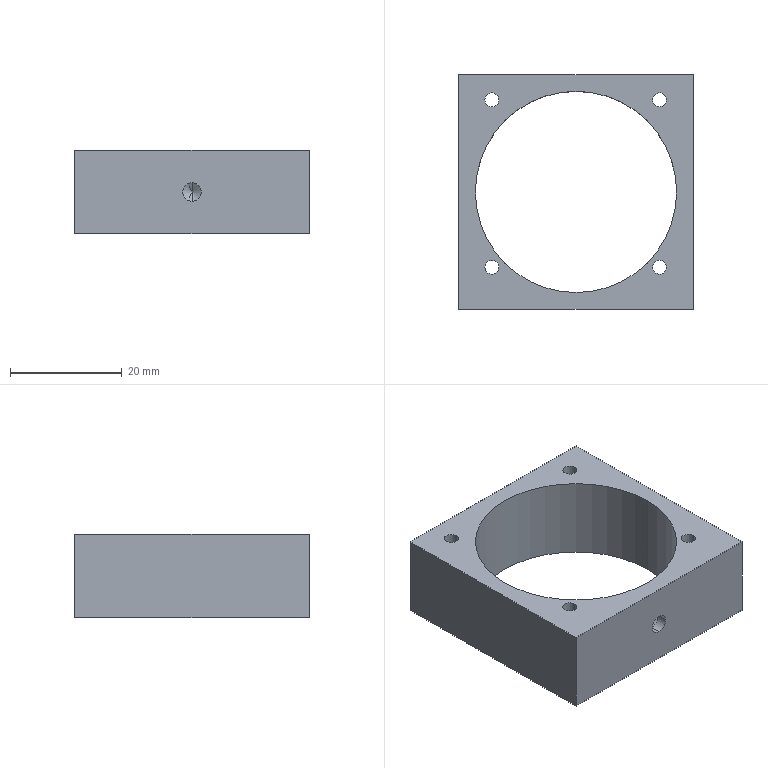Part | STEP file | custom lens barrel.step.STEP.STEP.STEP-260.STEP | 1 solid | 20 faces | box 42 x 42 x 15 mm | volume 10879 mm3 | cylinder 12 | plane 6 | cone 2 | commonest cylinder face diameters 2.5 x8 3.3 x2 36 x2
STEP:
#1=CARTESIAN_POINT('',(0.,-19.2,9.15));
#2=VERTEX_POINT('',#1);
#3=CARTESIAN_POINT('',(0.,-21.,9.15));
#4=VERTEX_POINT('',#3);
#5=CARTESIAN_POINT('',(0.,-21.,9.15));
#6=DIRECTION('',(0.,-1.,0.));
#7=VECTOR('',#6,1000.);
#8=LINE('',#5,#7);
#9=EDGE_CURVE('',#2,#4,#8,.T.);
#10=ORIENTED_EDGE('',*,*,#9,.F.);
#11=CARTESIAN_POINT('',(0.,-19.2,5.85));
#12=VERTEX_POINT('',#11);
#13=CARTESIAN_POINT('',(0.,-19.2,7.5));
#14=DIRECTION('',(0.,-1.,0.));
#15=DIRECTION('',(0.,0.,-1.));
#16=AXIS2_PLACEMENT_3D('',#13,#14,#15);
#17=CIRCLE('',#16,1.65);
#18=EDGE_CURVE('',#12,#2,#17,.T.);
#19=ORIENTED_EDGE('',*,*,#18,.F.);
#20=CARTESIAN_POINT('',(0.,-21.,5.85));
#21=VERTEX_POINT('',#20);
#22=CARTESIAN_POINT('',(0.,-21.,5.85));
#23=DIRECTION('',(0.,-1.,0.));
#24=VECTOR('',#23,1000.);
#25=LINE('',#22,#24);
#26=EDGE_CURVE('',#12,#21,#25,.T.);
#27=ORIENTED_EDGE('',*,*,#26,.T.);
#28=CARTESIAN_POINT('',(0.,-21.,7.5));
#29=DIRECTION('',(0.,-1.,0.));
#30=DIRECTION('',(0.,0.,-1.));
#31=AXIS2_PLACEMENT_3D('',#28,#29,#30);
#32=CIRCLE('',#31,1.65);
#33=EDGE_CURVE('',#21,#4,#32,.T.);
#34=ORIENTED_EDGE('',*,*,#33,.T.);
#35=EDGE_LOOP('',(#10,#19,#27,#34));
#36=FACE_OUTER_BOUND('',#35,.T.);
#37=CARTESIAN_POINT('',(0.,-21.,7.5));
#38=DIRECTION('',(0.,-1.,0.));
#39=DIRECTION('',(0.,0.,-1.));
#40=AXIS2_PLACEMENT_3D('',#37,#38,#39);
#41=CYLINDRICAL_SURFACE('',#40,1.65);
#42=ADVANCED_FACE('',(#36),#41,.F.);
#43=CARTESIAN_POINT('',(0.,-18.209,7.5));
#44=VERTEX_POINT('',#43);
#45=CARTESIAN_POINT('',(0.,-19.2,9.15));
#46=DIRECTION('',(0.,-0.515,0.8572));
#47=VECTOR('',#46,1000.);
#48=LINE('',#45,#47);
#49=EDGE_CURVE('',#44,#2,#48,.T.);
#50=ORIENTED_EDGE('',*,*,#49,.F.);
#51=CARTESIAN_POINT('',(0.,-19.2,5.85));
#52=DIRECTION('',(0.,-0.515,-0.8572));
#53=VECTOR('',#52,1000.);
#54=LINE('',#51,#53);
#55=EDGE_CURVE('',#44,#12,#54,.T.);
#56=ORIENTED_EDGE('',*,*,#55,.T.);
#57=ORIENTED_EDGE('',*,*,#18,.T.);
#58=EDGE_LOOP('',(#50,#56,#57));
#59=FACE_OUTER_BOUND('',#58,.T.);
#60=CARTESIAN_POINT('',(0.,-19.2,7.5));
#61=DIRECTION('',(0.,-1.,0.));
#62=DIRECTION('',(0.,0.,-1.));
#63=AXIS2_PLACEMENT_3D('',#60,#61,#62);
#64=CONICAL_SURFACE('',#63,1.65,1.03);
#65=ADVANCED_FACE('',(#59),#64,.F.);
#66=CARTESIAN_POINT('',(-16.304,16.486,0.));
#67=VERTEX_POINT('',#66);
#68=CARTESIAN_POINT('',(-16.304,16.486,15.));
#69=VERTEX_POINT('',#68);
#70=CARTESIAN_POINT('',(-16.304,16.486,15.));
#71=DIRECTION('',(0.,0.,1.));
#72=VECTOR('',#71,1000.);
#73=LINE('',#70,#72);
#74=EDGE_CURVE('',#67,#69,#73,.T.);
#75=ORIENTED_EDGE('',*,*,#74,.F.);
#76=CARTESIAN_POINT('',(-13.804,16.486,0.));
#77=VERTEX_POINT('',#76);
#78=CARTESIAN_POINT('',(-15.054,16.486,0.));
#79=DIRECTION('',(0.,0.,1.));
#80=DIRECTION('',(1.,0.,0.));
#81=AXIS2_PLACEMENT_3D('',#78,#79,#80);
#82=CIRCLE('',#81,1.25);
#83=EDGE_CURVE('',#77,#67,#82,.T.);
#84=ORIENTED_EDGE('',*,*,#83,.F.);
#85=CARTESIAN_POINT('',(-13.804,16.486,15.));
#86=VERTEX_POINT('',#85);
#87=CARTESIAN_POINT('',(-13.804,16.486,15.));
#88=DIRECTION('',(0.,0.,1.));
#89=VECTOR('',#88,1000.);
#90=LINE('',#87,#89);
#91=EDGE_CURVE('',#77,#86,#90,.T.);
#92=ORIENTED_EDGE('',*,*,#91,.T.);
#93=CARTESIAN_POINT('',(-15.054,16.486,15.));
#94=DIRECTION('',(0.,0.,1.));
#95=DIRECTION('',(1.,0.,0.));
#96=AXIS2_PLACEMENT_3D('',#93,#94,#95);
#97=CIRCLE('',#96,1.25);
#98=EDGE_CURVE('',#86,#69,#97,.T.);
#99=ORIENTED_EDGE('',*,*,#98,.T.);
#100=EDGE_LOOP('',(#75,#84,#92,#99));
#101=FACE_OUTER_BOUND('',#100,.T.);
#102=CARTESIAN_POINT('',(-15.054,16.486,15.));
#103=DIRECTION('',(0.,0.,1.));
#104=DIRECTION('',(1.,0.,0.));
#105=AXIS2_PLACEMENT_3D('',#102,#103,#104);
#106=CYLINDRICAL_SURFACE('',#105,1.25);
#107=ADVANCED_FACE('',(#101),#106,.F.);
#108=CARTESIAN_POINT('',(13.7,16.486,0.));
#109=VERTEX_POINT('',#108);
#110=CARTESIAN_POINT('',(13.7,16.486,15.));
#111=VERTEX_POINT('',#110);
#112=CARTESIAN_POINT('',(13.7,16.486,15.));
#113=DIRECTION('',(0.,0.,1.));
#114=VECTOR('',#113,1000.);
#115=LINE('',#112,#114);
#116=EDGE_CURVE('',#109,#111,#115,.T.);
#117=ORIENTED_EDGE('',*,*,#116,.F.);
#118=CARTESIAN_POINT('',(16.2,16.486,0.));
#119=VERTEX_POINT('',#118);
#120=CARTESIAN_POINT('',(14.95,16.486,0.));
#121=DIRECTION('',(0.,0.,1.));
#122=DIRECTION('',(1.,0.,0.));
#123=AXIS2_PLACEMENT_3D('',#120,#121,#122);
#124=CIRCLE('',#123,1.25);
#125=EDGE_CURVE('',#119,#109,#124,.T.);
#126=ORIENTED_EDGE('',*,*,#125,.F.);
#127=CARTESIAN_POINT('',(16.2,16.486,15.));
#128=VERTEX_POINT('',#127);
#129=CARTESIAN_POINT('',(16.2,16.486,15.));
#130=DIRECTION('',(0.,0.,1.));
#131=VECTOR('',#130,1000.);
#132=LINE('',#129,#131);
#133=EDGE_CURVE('',#119,#128,#132,.T.);
#134=ORIENTED_EDGE('',*,*,#133,.T.);
#135=CARTESIAN_POINT('',(14.95,16.486,15.));
#136=DIRECTION('',(0.,0.,1.));
#137=DIRECTION('',(1.,0.,0.));
#138=AXIS2_PLACEMENT_3D('',#135,#136,#137);
#139=CIRCLE('',#138,1.25);
#140=EDGE_CURVE('',#128,#111,#139,.T.);
#141=ORIENTED_EDGE('',*,*,#140,.T.);
#142=EDGE_LOOP('',(#117,#126,#134,#141));
#143=FACE_OUTER_BOUND('',#142,.T.);
#144=CARTESIAN_POINT('',(14.95,16.486,15.));
#145=DIRECTION('',(0.,0.,1.));
#146=DIRECTION('',(1.,0.,0.));
#147=AXIS2_PLACEMENT_3D('',#144,#145,#146);
#148=CYLINDRICAL_SURFACE('',#147,1.25);
#149=ADVANCED_FACE('',(#143),#148,.F.);
#150=CARTESIAN_POINT('',(13.7,-13.48,0.));
#151=VERTEX_POINT('',#150);
#152=CARTESIAN_POINT('',(13.7,-13.48,15.));
#153=VERTEX_POINT('',#152);
#154=CARTESIAN_POINT('',(13.7,-13.48,15.));
#155=DIRECTION('',(0.,0.,1.));
#156=VECTOR('',#155,1000.);
#157=LINE('',#154,#156);
#158=EDGE_CURVE('',#151,#153,#157,.T.);
#159=ORIENTED_EDGE('',*,*,#158,.F.);
#160=CARTESIAN_POINT('',(16.2,-13.48,0.));
#161=VERTEX_POINT('',#160);
#162=CARTESIAN_POINT('',(14.95,-13.48,0.));
#163=DIRECTION('',(0.,0.,1.));
#164=DIRECTION('',(1.,0.,0.));
#165=AXIS2_PLACEMENT_3D('',#162,#163,#164);
#166=CIRCLE('',#165,1.25);
#167=EDGE_CURVE('',#161,#151,#166,.T.);
#168=ORIENTED_EDGE('',*,*,#167,.F.);
#169=CARTESIAN_POINT('',(16.2,-13.48,15.));
#170=VERTEX_POINT('',#169);
#171=CARTESIAN_POINT('',(16.2,-13.48,15.));
#172=DIRECTION('',(0.,0.,1.));
#173=VECTOR('',#172,1000.);
#174=LINE('',#171,#173);
#175=EDGE_CURVE('',#161,#170,#174,.T.);
#176=ORIENTED_EDGE('',*,*,#175,.T.);
#177=CARTESIAN_POINT('',(14.95,-13.48,15.));
#178=DIRECTION('',(0.,0.,1.));
#179=DIRECTION('',(1.,0.,0.));
#180=AXIS2_PLACEMENT_3D('',#177,#178,#179);
#181=CIRCLE('',#180,1.25);
#182=EDGE_CURVE('',#170,#153,#181,.T.);
#183=ORIENTED_EDGE('',*,*,#182,.T.);
#184=EDGE_LOOP('',(#159,#168,#176,#183));
#185=FACE_OUTER_BOUND('',#184,.T.);
#186=CARTESIAN_POINT('',(14.95,-13.48,15.));
#187=DIRECTION('',(0.,0.,1.));
#188=DIRECTION('',(1.,0.,0.));
#189=AXIS2_PLACEMENT_3D('',#186,#187,#188);
#190=CYLINDRICAL_SURFACE('',#189,1.25);
#191=ADVANCED_FACE('',(#185),#190,.F.);
#192=CARTESIAN_POINT('',(-16.304,-13.48,0.));
#193=VERTEX_POINT('',#192);
#194=CARTESIAN_POINT('',(-16.304,-13.48,15.));
#195=VERTEX_POINT('',#194);
#196=CARTESIAN_POINT('',(-16.304,-13.48,15.));
#197=DIRECTION('',(0.,0.,1.));
#198=VECTOR('',#197,1000.);
#199=LINE('',#196,#198);
#200=EDGE_CURVE('',#193,#195,#199,.T.);
#201=ORIENTED_EDGE('',*,*,#200,.F.);
#202=CARTESIAN_POINT('',(-13.804,-13.48,0.));
#203=VERTEX_POINT('',#202);
#204=CARTESIAN_POINT('',(-15.054,-13.48,0.));
#205=DIRECTION('',(0.,0.,1.));
#206=DIRECTION('',(1.,0.,0.));
#207=AXIS2_PLACEMENT_3D('',#204,#205,#206);
#208=CIRCLE('',#207,1.25);
#209=EDGE_CURVE('',#203,#193,#208,.T.);
#210=ORIENTED_EDGE('',*,*,#209,.F.);
#211=CARTESIAN_POINT('',(-13.804,-13.48,15.));
#212=VERTEX_POINT('',#211);
#213=CARTESIAN_POINT('',(-13.804,-13.48,15.));
#214=DIRECTION('',(0.,0.,1.));
#215=VECTOR('',#214,1000.);
#216=LINE('',#213,#215);
#217=EDGE_CURVE('',#203,#212,#216,.T.);
#218=ORIENTED_EDGE('',*,*,#217,.T.);
#219=CARTESIAN_POINT('',(-15.054,-13.48,15.));
#220=DIRECTION('',(0.,0.,1.));
#221=DIRECTION('',(1.,0.,0.));
#222=AXIS2_PLACEMENT_3D('',#219,#220,#221);
#223=CIRCLE('',#222,1.25);
#224=EDGE_CURVE('',#212,#195,#223,.T.);
#225=ORIENTED_EDGE('',*,*,#224,.T.);
#226=EDGE_LOOP('',(#201,#210,#218,#225));
#227=FACE_OUTER_BOUND('',#226,.T.);
#228=CARTESIAN_POINT('',(-15.054,-13.48,15.));
#229=DIRECTION('',(0.,0.,1.));
#230=DIRECTION('',(1.,0.,0.));
#231=AXIS2_PLACEMENT_3D('',#228,#229,#230);
#232=CYLINDRICAL_SURFACE('',#231,1.25);
#233=ADVANCED_FACE('',(#227),#232,.F.);
#234=CARTESIAN_POINT('',(-18.,0.,0.));
#235=VERTEX_POINT('',#234);
#236=CARTESIAN_POINT('',(18.,0.,0.));
#237=VERTEX_POINT('',#236);
#238=CARTESIAN_POINT('',(0.,0.,0.));
#239=DIRECTION('',(0.,0.,1.));
#240=DIRECTION('',(1.,0.,0.));
#241=AXIS2_PLACEMENT_3D('',#238,#239,#240);
#242=CIRCLE('',#241,18.);
#243=EDGE_CURVE('',#235,#237,#242,.T.);
#244=ORIENTED_EDGE('',*,*,#243,.T.);
#245=CARTESIAN_POINT('',(0.,0.,0.));
#246=DIRECTION('',(0.,0.,1.));
#247=DIRECTION('',(1.,0.,0.));
#248=AXIS2_PLACEMENT_3D('',#245,#246,#247);
#249=CIRCLE('',#248,18.);
#250=EDGE_CURVE('',#237,#235,#249,.T.);
#251=ORIENTED_EDGE('',*,*,#250,.T.);
#252=EDGE_LOOP('',(#244,#251));
#253=FACE_BOUND('',#252,.T.);
#254=ORIENTED_EDGE('',*,*,#209,.T.);
#255=CARTESIAN_POINT('',(-15.054,-13.48,0.));
#256=DIRECTION('',(0.,0.,1.));
#257=DIRECTION('',(1.,0.,0.));
#258=AXIS2_PLACEMENT_3D('',#255,#256,#257);
#259=CIRCLE('',#258,1.25);
#260=EDGE_CURVE('',#193,#203,#259,.T.);
#261=ORIENTED_EDGE('',*,*,#260,.T.);
#262=EDGE_LOOP('',(#254,#261));
#263=FACE_BOUND('',#262,.T.);
#264=ORIENTED_EDGE('',*,*,#167,.T.);
#265=CARTESIAN_POINT('',(14.95,-13.48,0.));
#266=DIRECTION('',(0.,0.,1.));
#267=DIRECTION('',(1.,0.,0.));
#268=AXIS2_PLACEMENT_3D('',#265,#266,#267);
#269=CIRCLE('',#268,1.25);
#270=EDGE_CURVE('',#151,#161,#269,.T.);
#271=ORIENTED_EDGE('',*,*,#270,.T.);
#272=EDGE_LOOP('',(#264,#271));
#273=FACE_BOUND('',#272,.T.);
#274=ORIENTED_EDGE('',*,*,#125,.T.);
#275=CARTESIAN_POINT('',(14.95,16.486,0.));
#276=DIRECTION('',(0.,0.,1.));
#277=DIRECTION('',(1.,0.,0.));
#278=AXIS2_PLACEMENT_3D('',#275,#276,#277);
#279=CIRCLE('',#278,1.25);
#280=EDGE_CURVE('',#109,#119,#279,.T.);
#281=ORIENTED_EDGE('',*,*,#280,.T.);
#282=EDGE_LOOP('',(#274,#281));
#283=FACE_BOUND('',#282,.T.);
#284=ORIENTED_EDGE('',*,*,#83,.T.);
#285=CARTESIAN_POINT('',(-15.054,16.486,0.));
#286=DIRECTION('',(0.,0.,1.));
#287=DIRECTION('',(1.,0.,0.));
#288=AXIS2_PLACEMENT_3D('',#285,#286,#287);
#289=CIRCLE('',#288,1.25);
#290=EDGE_CURVE('',#67,#77,#289,.T.);
#291=ORIENTED_EDGE('',*,*,#290,.T.);
#292=EDGE_LOOP('',(#284,#291));
#293=FACE_BOUND('',#292,.T.);
#294=CARTESIAN_POINT('',(21.,21.,0.));
#295=VERTEX_POINT('',#294);
#296=CARTESIAN_POINT('',(21.,-21.,0.));
#297=VERTEX_POINT('',#296);
#298=CARTESIAN_POINT('',(21.,0.,0.));
#299=DIRECTION('',(0.,-1.,0.));
#300=VECTOR('',#299,1000.);
#301=LINE('',#298,#300);
#302=EDGE_CURVE('',#295,#297,#301,.T.);
#303=ORIENTED_EDGE('',*,*,#302,.T.);
#304=CARTESIAN_POINT('',(-21.,-21.,0.));
#305=VERTEX_POINT('',#304);
#306=CARTESIAN_POINT('',(0.,-21.,0.));
#307=DIRECTION('',(1.,0.,0.));
#308=VECTOR('',#307,1000.);
#309=LINE('',#306,#308);
#310=EDGE_CURVE('',#305,#297,#309,.T.);
#311=ORIENTED_EDGE('',*,*,#310,.F.);
#312=CARTESIAN_POINT('',(-21.,21.,0.));
#313=VERTEX_POINT('',#312);
#314=CARTESIAN_POINT('',(-21.,0.,0.));
#315=DIRECTION('',(0.,-1.,0.));
#316=VECTOR('',#315,1000.);
#317=LINE('',#314,#316);
#318=EDGE_CURVE('',#313,#305,#317,.T.);
#319=ORIENTED_EDGE('',*,*,#318,.F.);
#320=CARTESIAN_POINT('',(0.,21.,0.));
#321=DIRECTION('',(1.,0.,0.));
#322=VECTOR('',#321,1000.);
#323=LINE('',#320,#322);
#324=EDGE_CURVE('',#313,#295,#323,.T.);
#325=ORIENTED_EDGE('',*,*,#324,.T.);
#326=EDGE_LOOP('',(#303,#311,#319,#325));
#327=FACE_OUTER_BOUND('',#326,.T.);
#328=CARTESIAN_POINT('',(0.,0.,0.));
#329=DIRECTION('',(0.,0.,1.));
#330=DIRECTION('',(1.,0.,0.));
#331=AXIS2_PLACEMENT_3D('',#328,#329,#330);
#332=PLANE('',#331);
#333=ADVANCED_FACE('',(#253,#263,#273,#283,#293,#327),#332,.F.);
#334=CARTESIAN_POINT('',(-18.,0.,15.));
#335=VERTEX_POINT('',#334);
#336=CARTESIAN_POINT('',(18.,0.,15.));
#337=VERTEX_POINT('',#336);
#338=CARTESIAN_POINT('',(0.,0.,15.));
#339=DIRECTION('',(0.,0.,1.));
#340=DIRECTION('',(1.,0.,0.));
#341=AXIS2_PLACEMENT_3D('',#338,#339,#340);
#342=CIRCLE('',#341,18.);
#343=EDGE_CURVE('',#335,#337,#342,.T.);
#344=ORIENTED_EDGE('',*,*,#343,.F.);
#345=CARTESIAN_POINT('',(0.,0.,15.));
#346=DIRECTION('',(0.,0.,1.));
#347=DIRECTION('',(1.,0.,0.));
#348=AXIS2_PLACEMENT_3D('',#345,#346,#347);
#349=CIRCLE('',#348,18.);
#350=EDGE_CURVE('',#337,#335,#349,.T.);
#351=ORIENTED_EDGE('',*,*,#350,.F.);
#352=EDGE_LOOP('',(#344,#351));
#353=FACE_BOUND('',#352,.T.);
#354=ORIENTED_EDGE('',*,*,#224,.F.);
#355=CARTESIAN_POINT('',(-15.054,-13.48,15.));
#356=DIRECTION('',(0.,0.,1.));
#357=DIRECTION('',(1.,0.,0.));
#358=AXIS2_PLACEMENT_3D('',#355,#356,#357);
#359=CIRCLE('',#358,1.25);
#360=EDGE_CURVE('',#195,#212,#359,.T.);
#361=ORIENTED_EDGE('',*,*,#360,.F.);
#362=EDGE_LOOP('',(#354,#361));
#363=FACE_BOUND('',#362,.T.);
#364=ORIENTED_EDGE('',*,*,#182,.F.);
#365=CARTESIAN_POINT('',(14.95,-13.48,15.));
#366=DIRECTION('',(0.,0.,1.));
#367=DIRECTION('',(1.,0.,0.));
#368=AXIS2_PLACEMENT_3D('',#365,#366,#367);
#369=CIRCLE('',#368,1.25);
#370=EDGE_CURVE('',#153,#170,#369,.T.);
#371=ORIENTED_EDGE('',*,*,#370,.F.);
#372=EDGE_LOOP('',(#364,#371));
#373=FACE_BOUND('',#372,.T.);
#374=ORIENTED_EDGE('',*,*,#140,.F.);
#375=CARTESIAN_POINT('',(14.95,16.486,15.));
#376=DIRECTION('',(0.,0.,1.));
#377=DIRECTION('',(1.,0.,0.));
#378=AXIS2_PLACEMENT_3D('',#375,#376,#377);
#379=CIRCLE('',#378,1.25);
#380=EDGE_CURVE('',#111,#128,#379,.T.);
#381=ORIENTED_EDGE('',*,*,#380,.F.);
#382=EDGE_LOOP('',(#374,#381));
#383=FACE_BOUND('',#382,.T.);
#384=ORIENTED_EDGE('',*,*,#98,.F.);
#385=CARTESIAN_POINT('',(-15.054,16.486,15.));
#386=DIRECTION('',(0.,0.,1.));
#387=DIRECTION('',(1.,0.,0.));
#388=AXIS2_PLACEMENT_3D('',#385,#386,#387);
#389=CIRCLE('',#388,1.25);
#390=EDGE_CURVE('',#69,#86,#389,.T.);
#391=ORIENTED_EDGE('',*,*,#390,.F.);
#392=EDGE_LOOP('',(#384,#391));
#393=FACE_BOUND('',#392,.T.);
#394=CARTESIAN_POINT('',(21.,21.,15.));
#395=VERTEX_POINT('',#394);
#396=CARTESIAN_POINT('',(21.,-21.,15.));
#397=VERTEX_POINT('',#396);
#398=CARTESIAN_POINT('',(21.,0.,15.));
#399=DIRECTION('',(0.,-1.,0.));
#400=VECTOR('',#399,1000.);
#401=LINE('',#398,#400);
#402=EDGE_CURVE('',#395,#397,#401,.T.);
#403=ORIENTED_EDGE('',*,*,#402,.F.);
#404=CARTESIAN_POINT('',(-21.,21.,15.));
#405=VERTEX_POINT('',#404);
#406=CARTESIAN_POINT('',(0.,21.,15.));
#407=DIRECTION('',(1.,0.,0.));
#408=VECTOR('',#407,1000.);
#409=LINE('',#406,#408);
#410=EDGE_CURVE('',#405,#395,#409,.T.);
#411=ORIENTED_EDGE('',*,*,#410,.F.);
#412=CARTESIAN_POINT('',(-21.,-21.,15.));
#413=VERTEX_POINT('',#412);
#414=CARTESIAN_POINT('',(-21.,0.,15.));
#415=DIRECTION('',(0.,-1.,0.));
#416=VECTOR('',#415,1000.);
#417=LINE('',#414,#416);
#418=EDGE_CURVE('',#405,#413,#417,.T.);
#419=ORIENTED_EDGE('',*,*,#418,.T.);
#420=CARTESIAN_POINT('',(0.,-21.,15.));
#421=DIRECTION('',(1.,0.,0.));
#422=VECTOR('',#421,1000.);
#423=LINE('',#420,#422);
#424=EDGE_CURVE('',#413,#397,#423,.T.);
#425=ORIENTED_EDGE('',*,*,#424,.T.);
#426=EDGE_LOOP('',(#403,#411,#419,#425));
#427=FACE_OUTER_BOUND('',#426,.T.);
#428=CARTESIAN_POINT('',(0.,0.,15.));
#429=DIRECTION('',(0.,0.,1.));
#430=DIRECTION('',(1.,0.,0.));
#431=AXIS2_PLACEMENT_3D('',#428,#429,#430);
#432=PLANE('',#431);
#433=ADVANCED_FACE('',(#353,#363,#373,#383,#393,#427),#432,.T.);
#434=ORIENTED_EDGE('',*,*,#33,.F.);
#435=CARTESIAN_POINT('',(0.,-21.,7.5));
#436=DIRECTION('',(0.,-1.,0.));
#437=DIRECTION('',(0.,0.,-1.));
#438=AXIS2_PLACEMENT_3D('',#435,#436,#437);
#439=CIRCLE('',#438,1.65);
#440=EDGE_CURVE('',#4,#21,#439,.T.);
#441=ORIENTED_EDGE('',*,*,#440,.F.);
#442=EDGE_LOOP('',(#434,#441));
#443=FACE_BOUND('',#442,.T.);
#444=ORIENTED_EDGE('',*,*,#310,.T.);
#445=CARTESIAN_POINT('',(21.,-21.,15.));
#446=DIRECTION('',(0.,0.,-1.));
#447=VECTOR('',#446,1000.);
#448=LINE('',#445,#447);
#449=EDGE_CURVE('',#397,#297,#448,.T.);
#450=ORIENTED_EDGE('',*,*,#449,.F.);
#451=ORIENTED_EDGE('',*,*,#424,.F.);
#452=CARTESIAN_POINT('',(-21.,-21.,15.));
#453=DIRECTION('',(0.,0.,-1.));
#454=VECTOR('',#453,1000.);
#455=LINE('',#452,#454);
#456=EDGE_CURVE('',#413,#305,#455,.T.);
#457=ORIENTED_EDGE('',*,*,#456,.T.);
#458=EDGE_LOOP('',(#444,#450,#451,#457));
#459=FACE_OUTER_BOUND('',#458,.T.);
#460=CARTESIAN_POINT('',(0.,-21.,15.));
#461=DIRECTION('',(0.,1.,0.));
#462=DIRECTION('',(1.,0.,0.));
#463=AXIS2_PLACEMENT_3D('',#460,#461,#462);
#464=PLANE('',#463);
#465=ADVANCED_FACE('',(#443,#459),#464,.F.);
#466=CARTESIAN_POINT('',(18.,0.,15.));
#467=DIRECTION('',(0.,0.,-1.));
#468=VECTOR('',#467,1000.);
#469=LINE('',#466,#468);
#470=EDGE_CURVE('',#337,#237,#469,.T.);
#471=ORIENTED_EDGE('',*,*,#470,.F.);
#472=ORIENTED_EDGE('',*,*,#350,.T.);
#473=CARTESIAN_POINT('',(-18.,0.,15.));
#474=DIRECTION('',(0.,0.,-1.));
#475=VECTOR('',#474,1000.);
#476=LINE('',#473,#475);
#477=EDGE_CURVE('',#335,#235,#476,.T.);
#478=ORIENTED_EDGE('',*,*,#477,.T.);
#479=ORIENTED_EDGE('',*,*,#250,.F.);
#480=EDGE_LOOP('',(#471,#472,#478,#479));
#481=FACE_OUTER_BOUND('',#480,.T.);
#482=CARTESIAN_POINT('',(0.,0.,15.));
#483=DIRECTION('',(0.,0.,-1.));
#484=DIRECTION('',(-1.,0.,0.));
#485=AXIS2_PLACEMENT_3D('',#482,#483,#484);
#486=CYLINDRICAL_SURFACE('',#485,18.);
#487=ADVANCED_FACE('',(#481),#486,.F.);
#488=ORIENTED_EDGE('',*,*,#318,.T.);
#489=ORIENTED_EDGE('',*,*,#456,.F.);
#490=ORIENTED_EDGE('',*,*,#418,.F.);
#491=CARTESIAN_POINT('',(-21.,21.,15.));
#492=DIRECTION('',(0.,0.,-1.));
#493=VECTOR('',#492,1000.);
#494=LINE('',#491,#493);
#495=EDGE_CURVE('',#405,#313,#494,.T.);
#496=ORIENTED_EDGE('',*,*,#495,.T.);
#497=EDGE_LOOP('',(#488,#489,#490,#496));
#498=FACE_OUTER_BOUND('',#497,.T.);
#499=CARTESIAN_POINT('',(-21.,0.,15.));
#500=DIRECTION('',(1.,0.,0.));
#501=DIRECTION('',(0.,1.,0.));
#502=AXIS2_PLACEMENT_3D('',#499,#500,#501);
#503=PLANE('',#502);
#504=ADVANCED_FACE('',(#498),#503,.F.);
#505=ORIENTED_EDGE('',*,*,#324,.F.);
#506=ORIENTED_EDGE('',*,*,#495,.F.);
#507=ORIENTED_EDGE('',*,*,#410,.T.);
#508=CARTESIAN_POINT('',(21.,21.,15.));
#509=DIRECTION('',(0.,0.,-1.));
#510=VECTOR('',#509,1000.);
#511=LINE('',#508,#510);
#512=EDGE_CURVE('',#395,#295,#511,.T.);
#513=ORIENTED_EDGE('',*,*,#512,.T.);
#514=EDGE_LOOP('',(#505,#506,#507,#513));
#515=FACE_OUTER_BOUND('',#514,.T.);
#516=CARTESIAN_POINT('',(0.,21.,15.));
#517=DIRECTION('',(0.,1.,0.));
#518=DIRECTION('',(1.,0.,0.));
#519=AXIS2_PLACEMENT_3D('',#516,#517,#518);
#520=PLANE('',#519);
#521=ADVANCED_FACE('',(#515),#520,.T.);
#522=ORIENTED_EDGE('',*,*,#302,.F.);
#523=ORIENTED_EDGE('',*,*,#512,.F.);
#524=ORIENTED_EDGE('',*,*,#402,.T.);
#525=ORIENTED_EDGE('',*,*,#449,.T.);
#526=EDGE_LOOP('',(#522,#523,#524,#525));
#527=FACE_OUTER_BOUND('',#526,.T.);
#528=CARTESIAN_POINT('',(21.,0.,15.));
#529=DIRECTION('',(1.,0.,0.));
#530=DIRECTION('',(0.,1.,0.));
#531=AXIS2_PLACEMENT_3D('',#528,#529,#530);
#532=PLANE('',#531);
#533=ADVANCED_FACE('',(#527),#532,.T.);
#534=ORIENTED_EDGE('',*,*,#343,.T.);
#535=ORIENTED_EDGE('',*,*,#470,.T.);
#536=ORIENTED_EDGE('',*,*,#243,.F.);
#537=ORIENTED_EDGE('',*,*,#477,.F.);
#538=EDGE_LOOP('',(#534,#535,#536,#537));
#539=FACE_OUTER_BOUND('',#538,.T.);
#540=CARTESIAN_POINT('',(0.,0.,15.));
#541=DIRECTION('',(0.,0.,-1.));
#542=DIRECTION('',(-1.,0.,0.));
#543=AXIS2_PLACEMENT_3D('',#540,#541,#542);
#544=CYLINDRICAL_SURFACE('',#543,18.);
#545=ADVANCED_FACE('',(#539),#544,.F.);
#546=ORIENTED_EDGE('',*,*,#260,.F.);
#547=ORIENTED_EDGE('',*,*,#200,.T.);
#548=ORIENTED_EDGE('',*,*,#360,.T.);
#549=ORIENTED_EDGE('',*,*,#217,.F.);
#550=EDGE_LOOP('',(#546,#547,#548,#549));
#551=FACE_OUTER_BOUND('',#550,.T.);
#552=CARTESIAN_POINT('',(-15.054,-13.48,15.));
#553=DIRECTION('',(0.,0.,1.));
#554=DIRECTION('',(1.,0.,0.));
#555=AXIS2_PLACEMENT_3D('',#552,#553,#554);
#556=CYLINDRICAL_SURFACE('',#555,1.25);
#557=ADVANCED_FACE('',(#551),#556,.F.);
#558=ORIENTED_EDGE('',*,*,#270,.F.);
#559=ORIENTED_EDGE('',*,*,#158,.T.);
#560=ORIENTED_EDGE('',*,*,#370,.T.);
#561=ORIENTED_EDGE('',*,*,#175,.F.);
#562=EDGE_LOOP('',(#558,#559,#560,#561));
#563=FACE_OUTER_BOUND('',#562,.T.);
#564=CARTESIAN_POINT('',(14.95,-13.48,15.));
#565=DIRECTION('',(0.,0.,1.));
#566=DIRECTION('',(1.,0.,0.));
#567=AXIS2_PLACEMENT_3D('',#564,#565,#566);
#568=CYLINDRICAL_SURFACE('',#567,1.25);
#569=ADVANCED_FACE('',(#563),#568,.F.);
#570=ORIENTED_EDGE('',*,*,#280,.F.);
#571=ORIENTED_EDGE('',*,*,#116,.T.);
#572=ORIENTED_EDGE('',*,*,#380,.T.);
#573=ORIENTED_EDGE('',*,*,#133,.F.);
#574=EDGE_LOOP('',(#570,#571,#572,#573));
#575=FACE_OUTER_BOUND('',#574,.T.);
#576=CARTESIAN_POINT('',(14.95,16.486,15.));
#577=DIRECTION('',(0.,0.,1.));
#578=DIRECTION('',(1.,0.,0.));
#579=AXIS2_PLACEMENT_3D('',#576,#577,#578);
#580=CYLINDRICAL_SURFACE('',#579,1.25);
#581=ADVANCED_FACE('',(#575),#580,.F.);
#582=ORIENTED_EDGE('',*,*,#290,.F.);
#583=ORIENTED_EDGE('',*,*,#74,.T.);
#584=ORIENTED_EDGE('',*,*,#390,.T.);
#585=ORIENTED_EDGE('',*,*,#91,.F.);
#586=EDGE_LOOP('',(#582,#583,#584,#585));
#587=FACE_OUTER_BOUND('',#586,.T.);
#588=CARTESIAN_POINT('',(-15.054,16.486,15.));
#589=DIRECTION('',(0.,0.,1.));
#590=DIRECTION('',(1.,0.,0.));
#591=AXIS2_PLACEMENT_3D('',#588,#589,#590);
#592=CYLINDRICAL_SURFACE('',#591,1.25);
#593=ADVANCED_FACE('',(#587),#592,.F.);
#594=ORIENTED_EDGE('',*,*,#55,.F.);
#595=ORIENTED_EDGE('',*,*,#49,.T.);
#596=CARTESIAN_POINT('',(0.,-19.2,7.5));
#597=DIRECTION('',(0.,-1.,0.));
#598=DIRECTION('',(0.,0.,-1.));
#599=AXIS2_PLACEMENT_3D('',#596,#597,#598);
#600=CIRCLE('',#599,1.65);
#601=EDGE_CURVE('',#2,#12,#600,.T.);
#602=ORIENTED_EDGE('',*,*,#601,.T.);
#603=EDGE_LOOP('',(#594,#595,#602));
#604=FACE_OUTER_BOUND('',#603,.T.);
#605=CARTESIAN_POINT('',(0.,-19.2,7.5));
#606=DIRECTION('',(0.,-1.,0.));
#607=DIRECTION('',(0.,0.,-1.));
#608=AXIS2_PLACEMENT_3D('',#605,#606,#607);
#609=CONICAL_SURFACE('',#608,1.65,1.03);
#610=ADVANCED_FACE('',(#604),#609,.F.);
#611=ORIENTED_EDGE('',*,*,#601,.F.);
#612=ORIENTED_EDGE('',*,*,#9,.T.);
#613=ORIENTED_EDGE('',*,*,#440,.T.);
#614=ORIENTED_EDGE('',*,*,#26,.F.);
#615=EDGE_LOOP('',(#611,#612,#613,#614));
#616=FACE_OUTER_BOUND('',#615,.T.);
#617=CARTESIAN_POINT('',(0.,-21.,7.5));
#618=DIRECTION('',(0.,-1.,0.));
#619=DIRECTION('',(0.,0.,-1.));
#620=AXIS2_PLACEMENT_3D('',#617,#618,#619);
#621=CYLINDRICAL_SURFACE('',#620,1.65);
#622=ADVANCED_FACE('',(#616),#621,.F.);
#623=CLOSED_SHELL('',(#42,#65,#107,#149,#191,#233,#333,#433,#465,#487,#504,#521,#533,#545,#557,#569,#581,#593,#610,#622));
#624=MANIFOLD_SOLID_BREP('',#623);
#625=CARTESIAN_POINT('',(0.,0.,0.));
#626=DIRECTION('',(0.,0.,1.));
#627=DIRECTION('',(1.,0.,0.));
#628=AXIS2_PLACEMENT_3D('',#625,#626,#627);
#629=(LENGTH_UNIT()NAMED_UNIT(*)SI_UNIT(.MILLI.,.METRE.));
#630=UNCERTAINTY_MEASURE_WITH_UNIT(LENGTH_MEASURE(0.00001),#629,'','');
#631=(NAMED_UNIT(*)PLANE_ANGLE_UNIT()SI_UNIT($,.RADIAN.));
#632=(NAMED_UNIT(*)SI_UNIT($,.STERADIAN.)SOLID_ANGLE_UNIT());
#633=(GEOMETRIC_REPRESENTATION_CONTEXT(3)GLOBAL_UNCERTAINTY_ASSIGNED_CONTEXT((#630))GLOBAL_UNIT_ASSIGNED_CONTEXT((#629,#631,#632))REPRESENTATION_CONTEXT('',''));
#634=ADVANCED_BREP_SHAPE_REPRESENTATION('',(#624,#628),#633);